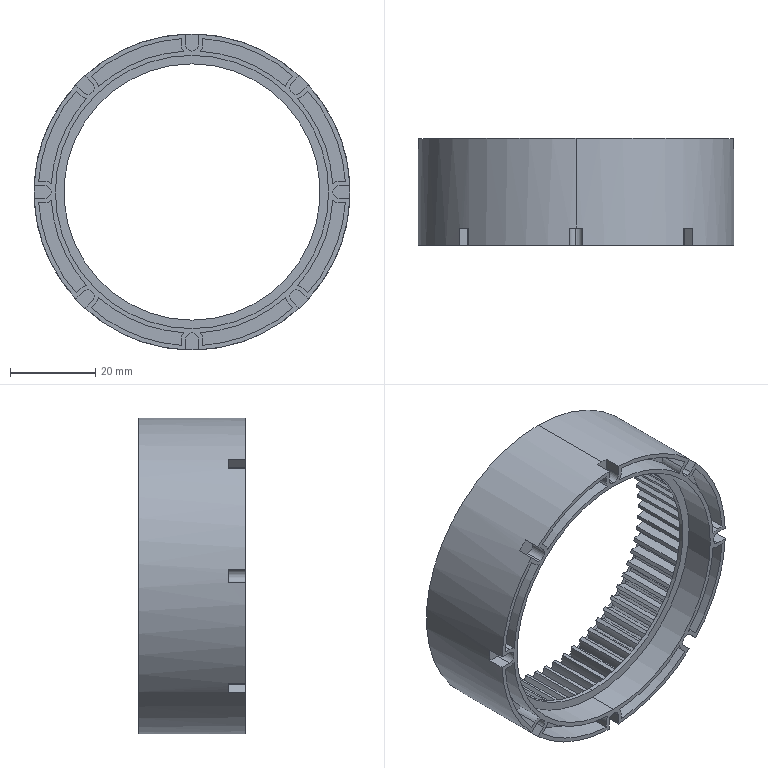Part | SolidWorks | features ICE 6, CirPattern 1, Extrusion 1 | 1 solid | 365 faces | box 74 x 25 x 74 mm | volume 22545 mm3 | cylinder 312 | plane 53 | commonest cylinder face diameters 25.6 x132 66 x72 61.498 x65 5 x16 3 x11 72 x8